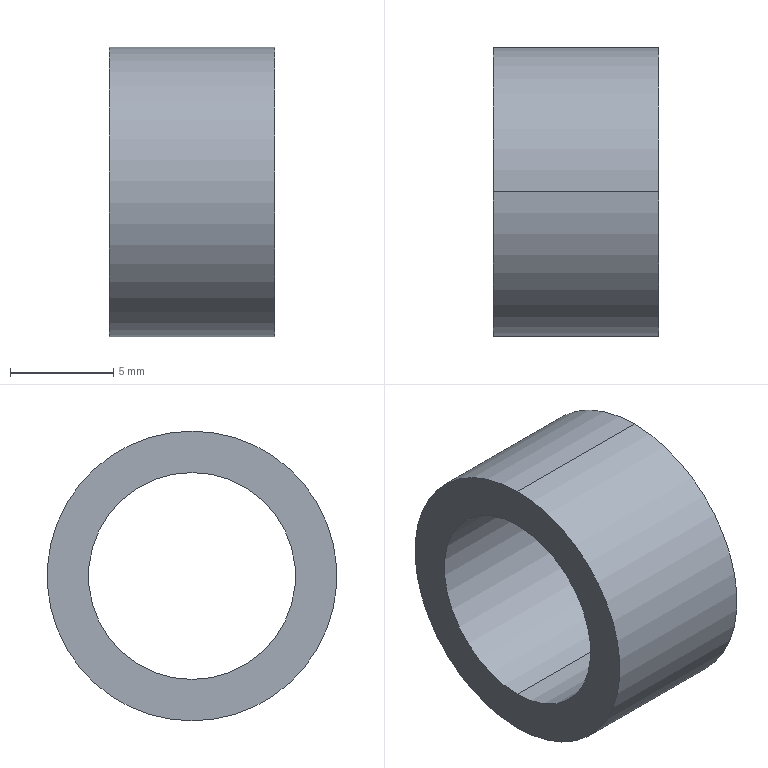Part | SolidWorks | features BaseBody 1 | 1 solid | 6 faces | box 8 x 14 x 14 mm | volume 603.186 mm3 | cylinder 4 | plane 2 | commonest cylinder face diameters 10 x2 14 x2
STEP:
#1=CARTESIAN_POINT('',(-4.,0.,-7.));
#2=VERTEX_POINT('',#1);
#3=CARTESIAN_POINT('',(-4.,0.,7.));
#4=VERTEX_POINT('',#3);
#5=CARTESIAN_POINT('',(-4.,0.,0.));
#6=DIRECTION('',(1.,0.,0.));
#7=DIRECTION('',(0.,0.,-1.));
#8=AXIS2_PLACEMENT_3D('',#5,#6,#7);
#9=CIRCLE('',#8,7.);
#10=EDGE_CURVE('',#2,#4,#9,.T.);
#11=ORIENTED_EDGE('',*,*,#10,.T.);
#12=CARTESIAN_POINT('',(4.,0.,7.));
#13=VERTEX_POINT('',#12);
#14=CARTESIAN_POINT('',(-4.,0.,7.));
#15=DIRECTION('',(1.,0.,0.));
#16=VECTOR('',#15,1000.);
#17=LINE('',#14,#16);
#18=EDGE_CURVE('',#4,#13,#17,.T.);
#19=ORIENTED_EDGE('',*,*,#18,.T.);
#20=CARTESIAN_POINT('',(4.,0.,-7.));
#21=VERTEX_POINT('',#20);
#22=CARTESIAN_POINT('',(4.,0.,0.));
#23=DIRECTION('',(-1.,0.,0.));
#24=DIRECTION('',(0.,0.,-1.));
#25=AXIS2_PLACEMENT_3D('',#22,#23,#24);
#26=CIRCLE('',#25,7.);
#27=EDGE_CURVE('',#13,#21,#26,.T.);
#28=ORIENTED_EDGE('',*,*,#27,.T.);
#29=CARTESIAN_POINT('',(-4.,0.,-7.));
#30=DIRECTION('',(1.,0.,0.));
#31=VECTOR('',#30,1000.);
#32=LINE('',#29,#31);
#33=EDGE_CURVE('',#2,#21,#32,.T.);
#34=ORIENTED_EDGE('',*,*,#33,.F.);
#35=EDGE_LOOP('',(#11,#19,#28,#34));
#36=FACE_OUTER_BOUND('',#35,.T.);
#37=CARTESIAN_POINT('',(-4.,0.,0.));
#38=DIRECTION('',(1.,0.,0.));
#39=DIRECTION('',(0.,0.,-1.));
#40=AXIS2_PLACEMENT_3D('',#37,#38,#39);
#41=CYLINDRICAL_SURFACE('',#40,7.);
#42=ADVANCED_FACE('',(#36),#41,.T.);
#43=CARTESIAN_POINT('',(-4.,0.,-5.));
#44=VERTEX_POINT('',#43);
#45=CARTESIAN_POINT('',(-4.,0.,5.));
#46=VERTEX_POINT('',#45);
#47=CARTESIAN_POINT('',(-4.,0.,0.));
#48=DIRECTION('',(-1.,0.,0.));
#49=DIRECTION('',(0.,0.,-1.));
#50=AXIS2_PLACEMENT_3D('',#47,#48,#49);
#51=CIRCLE('',#50,5.);
#52=EDGE_CURVE('',#44,#46,#51,.T.);
#53=ORIENTED_EDGE('',*,*,#52,.T.);
#54=CARTESIAN_POINT('',(4.,0.,5.));
#55=VERTEX_POINT('',#54);
#56=CARTESIAN_POINT('',(-5.,0.,5.));
#57=DIRECTION('',(1.,0.,0.));
#58=VECTOR('',#57,1000.);
#59=LINE('',#56,#58);
#60=EDGE_CURVE('',#46,#55,#59,.T.);
#61=ORIENTED_EDGE('',*,*,#60,.T.);
#62=CARTESIAN_POINT('',(4.,0.,-5.));
#63=VERTEX_POINT('',#62);
#64=CARTESIAN_POINT('',(4.,0.,0.));
#65=DIRECTION('',(-1.,0.,0.));
#66=DIRECTION('',(0.,0.,-1.));
#67=AXIS2_PLACEMENT_3D('',#64,#65,#66);
#68=CIRCLE('',#67,5.);
#69=EDGE_CURVE('',#63,#55,#68,.T.);
#70=ORIENTED_EDGE('',*,*,#69,.F.);
#71=CARTESIAN_POINT('',(-5.,0.,-5.));
#72=DIRECTION('',(1.,0.,0.));
#73=VECTOR('',#72,1000.);
#74=LINE('',#71,#73);
#75=EDGE_CURVE('',#44,#63,#74,.T.);
#76=ORIENTED_EDGE('',*,*,#75,.F.);
#77=EDGE_LOOP('',(#53,#61,#70,#76));
#78=FACE_OUTER_BOUND('',#77,.T.);
#79=CARTESIAN_POINT('',(-5.,0.,0.));
#80=DIRECTION('',(1.,0.,0.));
#81=DIRECTION('',(0.,0.,-1.));
#82=AXIS2_PLACEMENT_3D('',#79,#80,#81);
#83=CYLINDRICAL_SURFACE('',#82,5.);
#84=ADVANCED_FACE('',(#78),#83,.F.);
#85=ORIENTED_EDGE('',*,*,#18,.F.);
#86=CARTESIAN_POINT('',(-4.,0.,0.));
#87=DIRECTION('',(1.,0.,0.));
#88=DIRECTION('',(0.,0.,-1.));
#89=AXIS2_PLACEMENT_3D('',#86,#87,#88);
#90=CIRCLE('',#89,7.);
#91=EDGE_CURVE('',#4,#2,#90,.T.);
#92=ORIENTED_EDGE('',*,*,#91,.T.);
#93=ORIENTED_EDGE('',*,*,#33,.T.);
#94=CARTESIAN_POINT('',(4.,0.,0.));
#95=DIRECTION('',(-1.,0.,0.));
#96=DIRECTION('',(0.,0.,-1.));
#97=AXIS2_PLACEMENT_3D('',#94,#95,#96);
#98=CIRCLE('',#97,7.);
#99=EDGE_CURVE('',#21,#13,#98,.T.);
#100=ORIENTED_EDGE('',*,*,#99,.T.);
#101=EDGE_LOOP('',(#85,#92,#93,#100));
#102=FACE_OUTER_BOUND('',#101,.T.);
#103=CARTESIAN_POINT('',(-4.,0.,0.));
#104=DIRECTION('',(1.,0.,0.));
#105=DIRECTION('',(0.,0.,-1.));
#106=AXIS2_PLACEMENT_3D('',#103,#104,#105);
#107=CYLINDRICAL_SURFACE('',#106,7.);
#108=ADVANCED_FACE('',(#102),#107,.T.);
#109=ORIENTED_EDGE('',*,*,#52,.F.);
#110=CARTESIAN_POINT('',(-4.,0.,0.));
#111=DIRECTION('',(-1.,0.,0.));
#112=DIRECTION('',(0.,0.,-1.));
#113=AXIS2_PLACEMENT_3D('',#110,#111,#112);
#114=CIRCLE('',#113,5.);
#115=EDGE_CURVE('',#46,#44,#114,.T.);
#116=ORIENTED_EDGE('',*,*,#115,.F.);
#117=EDGE_LOOP('',(#109,#116));
#118=FACE_BOUND('',#117,.T.);
#119=ORIENTED_EDGE('',*,*,#10,.F.);
#120=ORIENTED_EDGE('',*,*,#91,.F.);
#121=EDGE_LOOP('',(#119,#120));
#122=FACE_OUTER_BOUND('',#121,.T.);
#123=CARTESIAN_POINT('',(-4.,0.,0.));
#124=DIRECTION('',(1.,0.,0.));
#125=DIRECTION('',(0.,0.,-1.));
#126=AXIS2_PLACEMENT_3D('',#123,#124,#125);
#127=PLANE('',#126);
#128=ADVANCED_FACE('',(#118,#122),#127,.F.);
#129=ORIENTED_EDGE('',*,*,#69,.T.);
#130=CARTESIAN_POINT('',(4.,0.,0.));
#131=DIRECTION('',(-1.,0.,0.));
#132=DIRECTION('',(0.,0.,-1.));
#133=AXIS2_PLACEMENT_3D('',#130,#131,#132);
#134=CIRCLE('',#133,5.);
#135=EDGE_CURVE('',#55,#63,#134,.T.);
#136=ORIENTED_EDGE('',*,*,#135,.T.);
#137=EDGE_LOOP('',(#129,#136));
#138=FACE_BOUND('',#137,.T.);
#139=ORIENTED_EDGE('',*,*,#99,.F.);
#140=ORIENTED_EDGE('',*,*,#27,.F.);
#141=EDGE_LOOP('',(#139,#140));
#142=FACE_OUTER_BOUND('',#141,.T.);
#143=CARTESIAN_POINT('',(4.,0.,0.));
#144=DIRECTION('',(1.,0.,0.));
#145=DIRECTION('',(0.,0.,-1.));
#146=AXIS2_PLACEMENT_3D('',#143,#144,#145);
#147=PLANE('',#146);
#148=ADVANCED_FACE('',(#138,#142),#147,.T.);
#149=ORIENTED_EDGE('',*,*,#60,.F.);
#150=ORIENTED_EDGE('',*,*,#115,.T.);
#151=ORIENTED_EDGE('',*,*,#75,.T.);
#152=ORIENTED_EDGE('',*,*,#135,.F.);
#153=EDGE_LOOP('',(#149,#150,#151,#152));
#154=FACE_OUTER_BOUND('',#153,.T.);
#155=CARTESIAN_POINT('',(-5.,0.,0.));
#156=DIRECTION('',(1.,0.,0.));
#157=DIRECTION('',(0.,0.,-1.));
#158=AXIS2_PLACEMENT_3D('',#155,#156,#157);
#159=CYLINDRICAL_SURFACE('',#158,5.);
#160=ADVANCED_FACE('',(#154),#159,.F.);
#161=CLOSED_SHELL('',(#42,#84,#108,#128,#148,#160));
#162=MANIFOLD_SOLID_BREP('',#161);
#163=CARTESIAN_POINT('',(0.,0.,0.));
#164=DIRECTION('',(0.,0.,1.));
#165=DIRECTION('',(1.,0.,0.));
#166=AXIS2_PLACEMENT_3D('',#163,#164,#165);
#167=(LENGTH_UNIT()NAMED_UNIT(*)SI_UNIT(.MILLI.,.METRE.));
#168=UNCERTAINTY_MEASURE_WITH_UNIT(LENGTH_MEASURE(0.00001),#167,'','');
#169=(NAMED_UNIT(*)PLANE_ANGLE_UNIT()SI_UNIT($,.RADIAN.));
#170=(NAMED_UNIT(*)SI_UNIT($,.STERADIAN.)SOLID_ANGLE_UNIT());
#171=(GEOMETRIC_REPRESENTATION_CONTEXT(3)GLOBAL_UNCERTAINTY_ASSIGNED_CONTEXT((#168))GLOBAL_UNIT_ASSIGNED_CONTEXT((#167,#169,#170))REPRESENTATION_CONTEXT('',''));
#172=ADVANCED_BREP_SHAPE_REPRESENTATION('',(#162,#166),#171);